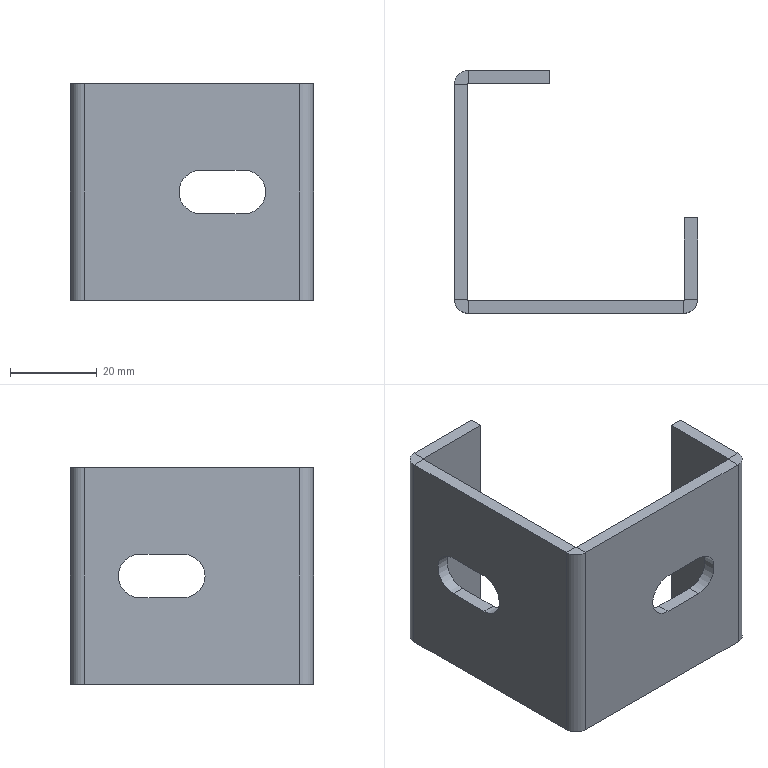Part | SolidWorks | features ICE 4, FlatPattern 1, SMBaseFlange 1, SheetMetal 1 | 1 solid | 39 faces | box 56 x 56 x 50 mm | volume 20650 mm3 | plane 28 | cylinder 11 | commonest cylinder face diameters 10 x5 0.4 x3 6.4 x3
STEP:
#1=CARTESIAN_POINT('',(3.,25.,0.));
#2=VERTEX_POINT('',#1);
#3=CARTESIAN_POINT('',(3.,30.,5.));
#4=VERTEX_POINT('',#3);
#5=CARTESIAN_POINT('',(3.,30.,0.));
#6=DIRECTION('',(-1.,0.,0.));
#7=DIRECTION('',(0.,-1.,0.));
#8=AXIS2_PLACEMENT_3D('',#5,#6,#7);
#9=CIRCLE('',#8,5.);
#10=EDGE_CURVE('',#2,#4,#9,.T.);
#11=ORIENTED_EDGE('',*,*,#10,.F.);
#12=CARTESIAN_POINT('',(0.,25.,0.));
#13=VERTEX_POINT('',#12);
#14=CARTESIAN_POINT('',(10.,25.,0.));
#15=DIRECTION('',(-1.,0.,0.));
#16=VECTOR('',#15,1000.);
#17=LINE('',#14,#16);
#18=EDGE_CURVE('',#2,#13,#17,.T.);
#19=ORIENTED_EDGE('',*,*,#18,.T.);
#20=CARTESIAN_POINT('',(0.,30.,5.));
#21=VERTEX_POINT('',#20);
#22=CARTESIAN_POINT('',(0.,30.,0.));
#23=DIRECTION('',(-1.,0.,0.));
#24=DIRECTION('',(0.,-1.,0.));
#25=AXIS2_PLACEMENT_3D('',#22,#23,#24);
#26=CIRCLE('',#25,5.);
#27=EDGE_CURVE('',#13,#21,#26,.T.);
#28=ORIENTED_EDGE('',*,*,#27,.T.);
#29=CARTESIAN_POINT('',(10.,30.,5.));
#30=DIRECTION('',(-1.,0.,0.));
#31=VECTOR('',#30,1000.);
#32=LINE('',#29,#31);
#33=EDGE_CURVE('',#4,#21,#32,.T.);
#34=ORIENTED_EDGE('',*,*,#33,.F.);
#35=EDGE_LOOP('',(#11,#19,#28,#34));
#36=FACE_OUTER_BOUND('',#35,.T.);
#37=CARTESIAN_POINT('',(10.,30.,0.));
#38=DIRECTION('',(-1.,0.,0.));
#39=DIRECTION('',(0.,-1.,0.));
#40=AXIS2_PLACEMENT_3D('',#37,#38,#39);
#41=CYLINDRICAL_SURFACE('',#40,5.);
#42=ADVANCED_FACE('',(#36),#41,.F.);
#43=CARTESIAN_POINT('',(52.8,0.,25.));
#44=VERTEX_POINT('',#43);
#45=CARTESIAN_POINT('',(52.8,3.,25.));
#46=VERTEX_POINT('',#45);
#47=CARTESIAN_POINT('',(52.8,0.,25.));
#48=DIRECTION('',(0.,1.,0.));
#49=VECTOR('',#48,1000.);
#50=LINE('',#47,#49);
#51=EDGE_CURVE('',#44,#46,#50,.T.);
#52=ORIENTED_EDGE('',*,*,#51,.F.);
#53=CARTESIAN_POINT('',(56.,3.2,25.));
#54=VERTEX_POINT('',#53);
#55=CARTESIAN_POINT('',(52.8,3.2,25.));
#56=DIRECTION('',(0.,0.,-1.));
#57=DIRECTION('',(1.,0.,0.));
#58=AXIS2_PLACEMENT_3D('',#55,#56,#57);
#59=CIRCLE('',#58,3.2);
#60=EDGE_CURVE('',#54,#44,#59,.T.);
#61=ORIENTED_EDGE('',*,*,#60,.F.);
#62=CARTESIAN_POINT('',(53.,3.2,25.));
#63=VERTEX_POINT('',#62);
#64=CARTESIAN_POINT('',(53.,3.2,25.));
#65=DIRECTION('',(1.,0.,0.));
#66=VECTOR('',#65,1000.);
#67=LINE('',#64,#66);
#68=EDGE_CURVE('',#63,#54,#67,.T.);
#69=ORIENTED_EDGE('',*,*,#68,.F.);
#70=CARTESIAN_POINT('',(52.8,3.2,25.));
#71=DIRECTION('',(0.,0.,-1.));
#72=DIRECTION('',(1.,0.,0.));
#73=AXIS2_PLACEMENT_3D('',#70,#71,#72);
#74=CIRCLE('',#73,0.2);
#75=EDGE_CURVE('',#63,#46,#74,.T.);
#76=ORIENTED_EDGE('',*,*,#75,.T.);
#77=EDGE_LOOP('',(#52,#61,#69,#76));
#78=FACE_OUTER_BOUND('',#77,.T.);
#79=CARTESIAN_POINT('',(52.8,0.,25.));
#80=DIRECTION('',(0.,0.,1.));
#81=DIRECTION('',(1.,0.,0.));
#82=AXIS2_PLACEMENT_3D('',#79,#80,#81);
#83=PLANE('',#82);
#84=ADVANCED_FACE('',(#78),#83,.T.);
#85=CARTESIAN_POINT('',(3.2,0.,25.));
#86=VERTEX_POINT('',#85);
#87=CARTESIAN_POINT('',(0.,0.,25.));
#88=DIRECTION('',(-1.,0.,0.));
#89=VECTOR('',#88,1000.);
#90=LINE('',#87,#89);
#91=EDGE_CURVE('',#44,#86,#90,.T.);
#92=ORIENTED_EDGE('',*,*,#91,.F.);
#93=ORIENTED_EDGE('',*,*,#51,.T.);
#94=CARTESIAN_POINT('',(3.2,3.,25.));
#95=VERTEX_POINT('',#94);
#96=CARTESIAN_POINT('',(0.,3.,25.));
#97=DIRECTION('',(-1.,0.,0.));
#98=VECTOR('',#97,1000.);
#99=LINE('',#96,#98);
#100=EDGE_CURVE('',#46,#95,#99,.T.);
#101=ORIENTED_EDGE('',*,*,#100,.T.);
#102=CARTESIAN_POINT('',(3.2,3.,25.));
#103=DIRECTION('',(0.,-1.,0.));
#104=VECTOR('',#103,1000.);
#105=LINE('',#102,#104);
#106=EDGE_CURVE('',#95,#86,#105,.T.);
#107=ORIENTED_EDGE('',*,*,#106,.T.);
#108=EDGE_LOOP('',(#92,#93,#101,#107));
#109=FACE_OUTER_BOUND('',#108,.T.);
#110=CARTESIAN_POINT('',(53.,3.2,25.));
#111=DIRECTION('',(0.,0.,1.));
#112=DIRECTION('',(1.,0.,0.));
#113=AXIS2_PLACEMENT_3D('',#110,#111,#112);
#114=PLANE('',#113);
#115=ADVANCED_FACE('',(#109),#114,.T.);
#116=CARTESIAN_POINT('',(56.,3.2,-25.));
#117=VERTEX_POINT('',#116);
#118=CARTESIAN_POINT('',(53.,3.2,-25.));
#119=VERTEX_POINT('',#118);
#120=CARTESIAN_POINT('',(56.,3.2,-25.));
#121=DIRECTION('',(-1.,0.,0.));
#122=VECTOR('',#121,1000.);
#123=LINE('',#120,#122);
#124=EDGE_CURVE('',#117,#119,#123,.T.);
#125=ORIENTED_EDGE('',*,*,#124,.F.);
#126=CARTESIAN_POINT('',(52.8,0.,-25.));
#127=VERTEX_POINT('',#126);
#128=CARTESIAN_POINT('',(52.8,3.2,-25.));
#129=DIRECTION('',(0.,0.,-1.));
#130=DIRECTION('',(1.,0.,0.));
#131=AXIS2_PLACEMENT_3D('',#128,#129,#130);
#132=CIRCLE('',#131,3.2);
#133=EDGE_CURVE('',#117,#127,#132,.T.);
#134=ORIENTED_EDGE('',*,*,#133,.T.);
#135=CARTESIAN_POINT('',(52.8,3.,-25.));
#136=VERTEX_POINT('',#135);
#137=CARTESIAN_POINT('',(52.8,3.,-25.));
#138=DIRECTION('',(0.,-1.,0.));
#139=VECTOR('',#138,1000.);
#140=LINE('',#137,#139);
#141=EDGE_CURVE('',#136,#127,#140,.T.);
#142=ORIENTED_EDGE('',*,*,#141,.F.);
#143=CARTESIAN_POINT('',(52.8,3.2,-25.));
#144=DIRECTION('',(0.,0.,-1.));
#145=DIRECTION('',(1.,0.,0.));
#146=AXIS2_PLACEMENT_3D('',#143,#144,#145);
#147=CIRCLE('',#146,0.2);
#148=EDGE_CURVE('',#119,#136,#147,.T.);
#149=ORIENTED_EDGE('',*,*,#148,.F.);
#150=EDGE_LOOP('',(#125,#134,#142,#149));
#151=FACE_OUTER_BOUND('',#150,.T.);
#152=CARTESIAN_POINT('',(56.,3.2,-25.));
#153=DIRECTION('',(0.,0.,-1.));
#154=DIRECTION('',(-1.,0.,0.));
#155=AXIS2_PLACEMENT_3D('',#152,#153,#154);
#156=PLANE('',#155);
#157=ADVANCED_FACE('',(#151),#156,.T.);
#158=CARTESIAN_POINT('',(56.,22.,-25.));
#159=VERTEX_POINT('',#158);
#160=CARTESIAN_POINT('',(56.,0.,-25.));
#161=DIRECTION('',(0.,-1.,0.));
#162=VECTOR('',#161,1000.);
#163=LINE('',#160,#162);
#164=EDGE_CURVE('',#159,#117,#163,.T.);
#165=ORIENTED_EDGE('',*,*,#164,.T.);
#166=ORIENTED_EDGE('',*,*,#124,.T.);
#167=CARTESIAN_POINT('',(53.,22.,-25.));
#168=VERTEX_POINT('',#167);
#169=CARTESIAN_POINT('',(53.,0.,-25.));
#170=DIRECTION('',(0.,-1.,0.));
#171=VECTOR('',#170,1000.);
#172=LINE('',#169,#171);
#173=EDGE_CURVE('',#168,#119,#172,.T.);
#174=ORIENTED_EDGE('',*,*,#173,.F.);
#175=CARTESIAN_POINT('',(53.,22.,-25.));
#176=DIRECTION('',(1.,0.,0.));
#177=VECTOR('',#176,1000.);
#178=LINE('',#175,#177);
#179=EDGE_CURVE('',#168,#159,#178,.T.);
#180=ORIENTED_EDGE('',*,*,#179,.T.);
#181=EDGE_LOOP('',(#165,#166,#174,#180));
#182=FACE_OUTER_BOUND('',#181,.T.);
#183=CARTESIAN_POINT('',(52.8,3.,-25.));
#184=DIRECTION('',(0.,0.,-1.));
#185=DIRECTION('',(-1.,0.,0.));
#186=AXIS2_PLACEMENT_3D('',#183,#184,#185);
#187=PLANE('',#186);
#188=ADVANCED_FACE('',(#182),#187,.T.);
#189=CARTESIAN_POINT('',(0.,3.2,25.));
#190=VERTEX_POINT('',#189);
#191=CARTESIAN_POINT('',(3.,3.2,25.));
#192=VERTEX_POINT('',#191);
#193=CARTESIAN_POINT('',(0.,3.2,25.));
#194=DIRECTION('',(1.,0.,0.));
#195=VECTOR('',#194,1000.);
#196=LINE('',#193,#195);
#197=EDGE_CURVE('',#190,#192,#196,.T.);
#198=ORIENTED_EDGE('',*,*,#197,.F.);
#199=CARTESIAN_POINT('',(3.2,3.2,25.));
#200=DIRECTION('',(0.,0.,-1.));
#201=DIRECTION('',(1.,0.,0.));
#202=AXIS2_PLACEMENT_3D('',#199,#200,#201);
#203=CIRCLE('',#202,3.2);
#204=EDGE_CURVE('',#86,#190,#203,.T.);
#205=ORIENTED_EDGE('',*,*,#204,.F.);
#206=ORIENTED_EDGE('',*,*,#106,.F.);
#207=CARTESIAN_POINT('',(3.2,3.2,25.));
#208=DIRECTION('',(0.,0.,-1.));
#209=DIRECTION('',(1.,0.,0.));
#210=AXIS2_PLACEMENT_3D('',#207,#208,#209);
#211=CIRCLE('',#210,0.2);
#212=EDGE_CURVE('',#95,#192,#211,.T.);
#213=ORIENTED_EDGE('',*,*,#212,.T.);
#214=EDGE_LOOP('',(#198,#205,#206,#213));
#215=FACE_OUTER_BOUND('',#214,.T.);
#216=CARTESIAN_POINT('',(0.,3.2,25.));
#217=DIRECTION('',(0.,0.,1.));
#218=DIRECTION('',(1.,0.,0.));
#219=AXIS2_PLACEMENT_3D('',#216,#217,#218);
#220=PLANE('',#219);
#221=ADVANCED_FACE('',(#215),#220,.T.);
#222=CARTESIAN_POINT('',(0.,52.8,25.));
#223=VERTEX_POINT('',#222);
#224=CARTESIAN_POINT('',(0.,56.,25.));
#225=DIRECTION('',(0.,1.,0.));
#226=VECTOR('',#225,1000.);
#227=LINE('',#224,#226);
#228=EDGE_CURVE('',#190,#223,#227,.T.);
#229=ORIENTED_EDGE('',*,*,#228,.F.);
#230=ORIENTED_EDGE('',*,*,#197,.T.);
#231=CARTESIAN_POINT('',(3.,52.8,25.));
#232=VERTEX_POINT('',#231);
#233=CARTESIAN_POINT('',(3.,56.,25.));
#234=DIRECTION('',(0.,1.,0.));
#235=VECTOR('',#234,1000.);
#236=LINE('',#233,#235);
#237=EDGE_CURVE('',#192,#232,#236,.T.);
#238=ORIENTED_EDGE('',*,*,#237,.T.);
#239=CARTESIAN_POINT('',(3.,52.8,25.));
#240=DIRECTION('',(-1.,0.,0.));
#241=VECTOR('',#240,1000.);
#242=LINE('',#239,#241);
#243=EDGE_CURVE('',#232,#223,#242,.T.);
#244=ORIENTED_EDGE('',*,*,#243,.T.);
#245=EDGE_LOOP('',(#229,#230,#238,#244));
#246=FACE_OUTER_BOUND('',#245,.T.);
#247=CARTESIAN_POINT('',(3.2,3.,25.));
#248=DIRECTION('',(0.,0.,1.));
#249=DIRECTION('',(1.,0.,0.));
#250=AXIS2_PLACEMENT_3D('',#247,#248,#249);
#251=PLANE('',#250);
#252=ADVANCED_FACE('',(#246),#251,.T.);
#253=CARTESIAN_POINT('',(3.2,0.,-25.));
#254=VERTEX_POINT('',#253);
#255=CARTESIAN_POINT('',(3.2,3.,-25.));
#256=VERTEX_POINT('',#255);
#257=CARTESIAN_POINT('',(3.2,0.,-25.));
#258=DIRECTION('',(0.,1.,0.));
#259=VECTOR('',#258,1000.);
#260=LINE('',#257,#259);
#261=EDGE_CURVE('',#254,#256,#260,.T.);
#262=ORIENTED_EDGE('',*,*,#261,.F.);
#263=CARTESIAN_POINT('',(0.,3.2,-25.));
#264=VERTEX_POINT('',#263);
#265=CARTESIAN_POINT('',(3.2,3.2,-25.));
#266=DIRECTION('',(0.,0.,-1.));
#267=DIRECTION('',(1.,0.,0.));
#268=AXIS2_PLACEMENT_3D('',#265,#266,#267);
#269=CIRCLE('',#268,3.2);
#270=EDGE_CURVE('',#254,#264,#269,.T.);
#271=ORIENTED_EDGE('',*,*,#270,.T.);
#272=CARTESIAN_POINT('',(3.,3.2,-25.));
#273=VERTEX_POINT('',#272);
#274=CARTESIAN_POINT('',(3.,3.2,-25.));
#275=DIRECTION('',(-1.,0.,0.));
#276=VECTOR('',#275,1000.);
#277=LINE('',#274,#276);
#278=EDGE_CURVE('',#273,#264,#277,.T.);
#279=ORIENTED_EDGE('',*,*,#278,.F.);
#280=CARTESIAN_POINT('',(3.2,3.2,-25.));
#281=DIRECTION('',(0.,0.,-1.));
#282=DIRECTION('',(1.,0.,0.));
#283=AXIS2_PLACEMENT_3D('',#280,#281,#282);
#284=CIRCLE('',#283,0.2);
#285=EDGE_CURVE('',#256,#273,#284,.T.);
#286=ORIENTED_EDGE('',*,*,#285,.F.);
#287=EDGE_LOOP('',(#262,#271,#279,#286));
#288=FACE_OUTER_BOUND('',#287,.T.);
#289=CARTESIAN_POINT('',(3.2,0.,-25.));
#290=DIRECTION('',(0.,0.,-1.));
#291=DIRECTION('',(-1.,0.,0.));
#292=AXIS2_PLACEMENT_3D('',#289,#290,#291);
#293=PLANE('',#292);
#294=ADVANCED_FACE('',(#288),#293,.T.);
#295=CARTESIAN_POINT('',(0.,0.,-25.));
#296=DIRECTION('',(-1.,0.,0.));
#297=VECTOR('',#296,1000.);
#298=LINE('',#295,#297);
#299=EDGE_CURVE('',#127,#254,#298,.T.);
#300=ORIENTED_EDGE('',*,*,#299,.T.);
#301=ORIENTED_EDGE('',*,*,#261,.T.);
#302=CARTESIAN_POINT('',(0.,3.,-25.));
#303=DIRECTION('',(-1.,0.,0.));
#304=VECTOR('',#303,1000.);
#305=LINE('',#302,#304);
#306=EDGE_CURVE('',#136,#256,#305,.T.);
#307=ORIENTED_EDGE('',*,*,#306,.F.);
#308=ORIENTED_EDGE('',*,*,#141,.T.);
#309=EDGE_LOOP('',(#300,#301,#307,#308));
#310=FACE_OUTER_BOUND('',#309,.T.);
#311=CARTESIAN_POINT('',(3.,3.2,-25.));
#312=DIRECTION('',(0.,0.,-1.));
#313=DIRECTION('',(-1.,0.,0.));
#314=AXIS2_PLACEMENT_3D('',#311,#312,#313);
#315=PLANE('',#314);
#316=ADVANCED_FACE('',(#310),#315,.T.);
#317=CARTESIAN_POINT('',(3.2,56.,25.));
#318=VERTEX_POINT('',#317);
#319=CARTESIAN_POINT('',(3.2,53.,25.));
#320=VERTEX_POINT('',#319);
#321=CARTESIAN_POINT('',(3.2,56.,25.));
#322=DIRECTION('',(0.,-1.,0.));
#323=VECTOR('',#322,1000.);
#324=LINE('',#321,#323);
#325=EDGE_CURVE('',#318,#320,#324,.T.);
#326=ORIENTED_EDGE('',*,*,#325,.F.);
#327=CARTESIAN_POINT('',(3.2,52.8,25.));
#328=DIRECTION('',(0.,0.,-1.));
#329=DIRECTION('',(1.,0.,0.));
#330=AXIS2_PLACEMENT_3D('',#327,#328,#329);
#331=CIRCLE('',#330,3.2);
#332=EDGE_CURVE('',#223,#318,#331,.T.);
#333=ORIENTED_EDGE('',*,*,#332,.F.);
#334=ORIENTED_EDGE('',*,*,#243,.F.);
#335=CARTESIAN_POINT('',(3.2,52.8,25.));
#336=DIRECTION('',(0.,0.,-1.));
#337=DIRECTION('',(1.,0.,0.));
#338=AXIS2_PLACEMENT_3D('',#335,#336,#337);
#339=CIRCLE('',#338,0.2);
#340=EDGE_CURVE('',#232,#320,#339,.T.);
#341=ORIENTED_EDGE('',*,*,#340,.T.);
#342=EDGE_LOOP('',(#326,#333,#334,#341));
#343=FACE_OUTER_BOUND('',#342,.T.);
#344=CARTESIAN_POINT('',(3.2,56.,25.));
#345=DIRECTION('',(0.,0.,1.));
#346=DIRECTION('',(1.,0.,0.));
#347=AXIS2_PLACEMENT_3D('',#344,#345,#346);
#348=PLANE('',#347);
#349=ADVANCED_FACE('',(#343),#348,.T.);
#350=CARTESIAN_POINT('',(22.,56.,25.));
#351=VERTEX_POINT('',#350);
#352=CARTESIAN_POINT('',(0.,56.,25.));
#353=DIRECTION('',(1.,0.,0.));
#354=VECTOR('',#353,1000.);
#355=LINE('',#352,#354);
#356=EDGE_CURVE('',#318,#351,#355,.T.);
#357=ORIENTED_EDGE('',*,*,#356,.F.);
#358=ORIENTED_EDGE('',*,*,#325,.T.);
#359=CARTESIAN_POINT('',(22.,53.,25.));
#360=VERTEX_POINT('',#359);
#361=CARTESIAN_POINT('',(0.,53.,25.));
#362=DIRECTION('',(1.,0.,0.));
#363=VECTOR('',#362,1000.);
#364=LINE('',#361,#363);
#365=EDGE_CURVE('',#320,#360,#364,.T.);
#366=ORIENTED_EDGE('',*,*,#365,.T.);
#367=CARTESIAN_POINT('',(22.,56.,25.));
#368=DIRECTION('',(0.,-1.,0.));
#369=VECTOR('',#368,1000.);
#370=LINE('',#367,#369);
#371=EDGE_CURVE('',#351,#360,#370,.T.);
#372=ORIENTED_EDGE('',*,*,#371,.F.);
#373=EDGE_LOOP('',(#357,#358,#366,#372));
#374=FACE_OUTER_BOUND('',#373,.T.);
#375=CARTESIAN_POINT('',(3.,52.8,25.));
#376=DIRECTION('',(0.,0.,1.));
#377=DIRECTION('',(1.,0.,0.));
#378=AXIS2_PLACEMENT_3D('',#375,#376,#377);
#379=PLANE('',#378);
#380=ADVANCED_FACE('',(#374),#379,.T.);
#381=CARTESIAN_POINT('',(0.,52.8,-25.));
#382=VERTEX_POINT('',#381);
#383=CARTESIAN_POINT('',(3.,52.8,-25.));
#384=VERTEX_POINT('',#383);
#385=CARTESIAN_POINT('',(0.,52.8,-25.));
#386=DIRECTION('',(1.,0.,0.));
#387=VECTOR('',#386,1000.);
#388=LINE('',#385,#387);
#389=EDGE_CURVE('',#382,#384,#388,.T.);
#390=ORIENTED_EDGE('',*,*,#389,.F.);
#391=CARTESIAN_POINT('',(3.2,56.,-25.));
#392=VERTEX_POINT('',#391);
#393=CARTESIAN_POINT('',(3.2,52.8,-25.));
#394=DIRECTION('',(0.,0.,-1.));
#395=DIRECTION('',(1.,0.,0.));
#396=AXIS2_PLACEMENT_3D('',#393,#394,#395);
#397=CIRCLE('',#396,3.2);
#398=EDGE_CURVE('',#382,#392,#397,.T.);
#399=ORIENTED_EDGE('',*,*,#398,.T.);
#400=CARTESIAN_POINT('',(3.2,53.,-25.));
#401=VERTEX_POINT('',#400);
#402=CARTESIAN_POINT('',(3.2,53.,-25.));
#403=DIRECTION('',(0.,1.,0.));
#404=VECTOR('',#403,1000.);
#405=LINE('',#402,#404);
#406=EDGE_CURVE('',#401,#392,#405,.T.);
#407=ORIENTED_EDGE('',*,*,#406,.F.);
#408=CARTESIAN_POINT('',(3.2,52.8,-25.));
#409=DIRECTION('',(0.,0.,-1.));
#410=DIRECTION('',(1.,0.,0.));
#411=AXIS2_PLACEMENT_3D('',#408,#409,#410);
#412=CIRCLE('',#411,0.2);
#413=EDGE_CURVE('',#384,#401,#412,.T.);
#414=ORIENTED_EDGE('',*,*,#413,.F.);
#415=EDGE_LOOP('',(#390,#399,#407,#414));
#416=FACE_OUTER_BOUND('',#415,.T.);
#417=CARTESIAN_POINT('',(0.,52.8,-25.));
#418=DIRECTION('',(0.,0.,-1.));
#419=DIRECTION('',(-1.,0.,0.));
#420=AXIS2_PLACEMENT_3D('',#417,#418,#419);
#421=PLANE('',#420);
#422=ADVANCED_FACE('',(#416),#421,.T.);
#423=CARTESIAN_POINT('',(0.,56.,-25.));
#424=DIRECTION('',(0.,1.,0.));
#425=VECTOR('',#424,1000.);
#426=LINE('',#423,#425);
#427=EDGE_CURVE('',#264,#382,#426,.T.);
#428=ORIENTED_EDGE('',*,*,#427,.T.);
#429=ORIENTED_EDGE('',*,*,#389,.T.);
#430=CARTESIAN_POINT('',(3.,56.,-25.));
#431=DIRECTION('',(0.,1.,0.));
#432=VECTOR('',#431,1000.);
#433=LINE('',#430,#432);
#434=EDGE_CURVE('',#273,#384,#433,.T.);
#435=ORIENTED_EDGE('',*,*,#434,.F.);
#436=ORIENTED_EDGE('',*,*,#278,.T.);
#437=EDGE_LOOP('',(#428,#429,#435,#436));
#438=FACE_OUTER_BOUND('',#437,.T.);
#439=CARTESIAN_POINT('',(3.2,53.,-25.));
#440=DIRECTION('',(0.,0.,-1.));
#441=DIRECTION('',(-1.,0.,0.));
#442=AXIS2_PLACEMENT_3D('',#439,#440,#441);
#443=PLANE('',#442);
#444=ADVANCED_FACE('',(#438),#443,.T.);
#445=CARTESIAN_POINT('',(22.,53.,-25.));
#446=VERTEX_POINT('',#445);
#447=CARTESIAN_POINT('',(0.,53.,-25.));
#448=DIRECTION('',(1.,0.,0.));
#449=VECTOR('',#448,1000.);
#450=LINE('',#447,#449);
#451=EDGE_CURVE('',#401,#446,#450,.T.);
#452=ORIENTED_EDGE('',*,*,#451,.T.);
#453=CARTESIAN_POINT('',(22.,53.,25.));
#454=DIRECTION('',(0.,0.,-1.));
#455=VECTOR('',#454,1000.);
#456=LINE('',#453,#455);
#457=EDGE_CURVE('',#360,#446,#456,.T.);
#458=ORIENTED_EDGE('',*,*,#457,.F.);
#459=ORIENTED_EDGE('',*,*,#365,.F.);
#460=CARTESIAN_POINT('',(3.2,53.,25.));
#461=DIRECTION('',(0.,0.,-1.));
#462=VECTOR('',#461,1000.);
#463=LINE('',#460,#462);
#464=EDGE_CURVE('',#320,#401,#463,.T.);
#465=ORIENTED_EDGE('',*,*,#464,.T.);
#466=EDGE_LOOP('',(#452,#458,#459,#465));
#467=FACE_OUTER_BOUND('',#466,.T.);
#468=CARTESIAN_POINT('',(0.,53.,25.));
#469=DIRECTION('',(0.,1.,0.));
#470=DIRECTION('',(0.,0.,1.));
#471=AXIS2_PLACEMENT_3D('',#468,#469,#470);
#472=PLANE('',#471);
#473=ADVANCED_FACE('',(#467),#472,.F.);
#474=CARTESIAN_POINT('',(22.,56.,-25.));
#475=VERTEX_POINT('',#474);
#476=CARTESIAN_POINT('',(22.,56.,-25.));
#477=DIRECTION('',(0.,-1.,0.));
#478=VECTOR('',#477,1000.);
#479=LINE('',#476,#478);
#480=EDGE_CURVE('',#475,#446,#479,.T.);
#481=ORIENTED_EDGE('',*,*,#480,.F.);
#482=CARTESIAN_POINT('',(22.,56.,25.));
#483=DIRECTION('',(0.,0.,-1.));
#484=VECTOR('',#483,1000.);
#485=LINE('',#482,#484);
#486=EDGE_CURVE('',#351,#475,#485,.T.);
#487=ORIENTED_EDGE('',*,*,#486,.F.);
#488=ORIENTED_EDGE('',*,*,#371,.T.);
#489=ORIENTED_EDGE('',*,*,#457,.T.);
#490=EDGE_LOOP('',(#481,#487,#488,#489));
#491=FACE_OUTER_BOUND('',#490,.T.);
#492=CARTESIAN_POINT('',(22.,56.,25.));
#493=DIRECTION('',(1.,0.,0.));
#494=DIRECTION('',(0.,0.,-1.));
#495=AXIS2_PLACEMENT_3D('',#492,#493,#494);
#496=PLANE('',#495);
#497=ADVANCED_FACE('',(#491),#496,.T.);
#498=CARTESIAN_POINT('',(0.,56.,-25.));
#499=DIRECTION('',(1.,0.,0.));
#500=VECTOR('',#499,1000.);
#501=LINE('',#498,#500);
#502=EDGE_CURVE('',#392,#475,#501,.T.);
#503=ORIENTED_EDGE('',*,*,#502,.F.);
#504=CARTESIAN_POINT('',(3.2,56.,25.));
#505=DIRECTION('',(0.,0.,-1.));
#506=VECTOR('',#505,1000.);
#507=LINE('',#504,#506);
#508=EDGE_CURVE('',#318,#392,#507,.T.);
#509=ORIENTED_EDGE('',*,*,#508,.F.);
#510=ORIENTED_EDGE('',*,*,#356,.T.);
#511=ORIENTED_EDGE('',*,*,#486,.T.);
#512=EDGE_LOOP('',(#503,#509,#510,#511));
#513=FACE_OUTER_BOUND('',#512,.T.);
#514=CARTESIAN_POINT('',(0.,56.,25.));
#515=DIRECTION('',(0.,1.,0.));
#516=DIRECTION('',(0.,0.,1.));
#517=AXIS2_PLACEMENT_3D('',#514,#515,#516);
#518=PLANE('',#517);
#519=ADVANCED_FACE('',(#513),#518,.T.);
#520=ORIENTED_EDGE('',*,*,#398,.F.);
#521=CARTESIAN_POINT('',(0.,52.8,25.));
#522=DIRECTION('',(0.,0.,-1.));
#523=VECTOR('',#522,1000.);
#524=LINE('',#521,#523);
#525=EDGE_CURVE('',#223,#382,#524,.T.);
#526=ORIENTED_EDGE('',*,*,#525,.F.);
#527=ORIENTED_EDGE('',*,*,#332,.T.);
#528=ORIENTED_EDGE('',*,*,#508,.T.);
#529=EDGE_LOOP('',(#520,#526,#527,#528));
#530=FACE_OUTER_BOUND('',#529,.T.);
#531=CARTESIAN_POINT('',(3.2,52.8,25.));
#532=DIRECTION('',(0.,0.,-1.));
#533=DIRECTION('',(-1.,0.,0.));
#534=AXIS2_PLACEMENT_3D('',#531,#532,#533);
#535=CYLINDRICAL_SURFACE('',#534,3.2);
#536=ADVANCED_FACE('',(#530),#535,.T.);
#537=CARTESIAN_POINT('',(0.,40.,5.));
#538=VERTEX_POINT('',#537);
#539=CARTESIAN_POINT('',(0.,40.,-5.));
#540=VERTEX_POINT('',#539);
#541=CARTESIAN_POINT('',(0.,40.,0.));
#542=DIRECTION('',(-1.,0.,0.));
#543=DIRECTION('',(0.,-1.,0.));
#544=AXIS2_PLACEMENT_3D('',#541,#542,#543);
#545=CIRCLE('',#544,5.);
#546=EDGE_CURVE('',#538,#540,#545,.T.);
#547=ORIENTED_EDGE('',*,*,#546,.F.);
#548=CARTESIAN_POINT('',(0.,40.,5.));
#549=DIRECTION('',(0.,1.,0.));
#550=VECTOR('',#549,1000.);
#551=LINE('',#548,#550);
#552=EDGE_CURVE('',#21,#538,#551,.T.);
#553=ORIENTED_EDGE('',*,*,#552,.F.);
#554=ORIENTED_EDGE('',*,*,#27,.F.);
#555=CARTESIAN_POINT('',(0.,30.,-5.));
#556=VERTEX_POINT('',#555);
#557=CARTESIAN_POINT('',(0.,30.,0.));
#558=DIRECTION('',(-1.,0.,0.));
#559=DIRECTION('',(0.,-1.,0.));
#560=AXIS2_PLACEMENT_3D('',#557,#558,#559);
#561=CIRCLE('',#560,5.);
#562=EDGE_CURVE('',#556,#13,#561,.T.);
#563=ORIENTED_EDGE('',*,*,#562,.F.);
#564=CARTESIAN_POINT('',(0.,40.,-5.));
#565=DIRECTION('',(0.,-1.,0.));
#566=VECTOR('',#565,1000.);
#567=LINE('',#564,#566);
#568=EDGE_CURVE('',#540,#556,#567,.T.);
#569=ORIENTED_EDGE('',*,*,#568,.F.);
#570=EDGE_LOOP('',(#547,#553,#554,#563,#569));
#571=FACE_BOUND('',#570,.T.);
#572=ORIENTED_EDGE('',*,*,#427,.F.);
#573=CARTESIAN_POINT('',(0.,3.2,25.));
#574=DIRECTION('',(0.,0.,-1.));
#575=VECTOR('',#574,1000.);
#576=LINE('',#573,#575);
#577=EDGE_CURVE('',#190,#264,#576,.T.);
#578=ORIENTED_EDGE('',*,*,#577,.F.);
#579=ORIENTED_EDGE('',*,*,#228,.T.);
#580=ORIENTED_EDGE('',*,*,#525,.T.);
#581=EDGE_LOOP('',(#572,#578,#579,#580));
#582=FACE_OUTER_BOUND('',#581,.T.);
#583=CARTESIAN_POINT('',(0.,56.,25.));
#584=DIRECTION('',(-1.,0.,0.));
#585=DIRECTION('',(0.,-1.,0.));
#586=AXIS2_PLACEMENT_3D('',#583,#584,#585);
#587=PLANE('',#586);
#588=ADVANCED_FACE('',(#571,#582),#587,.T.);
#589=ORIENTED_EDGE('',*,*,#270,.F.);
#590=CARTESIAN_POINT('',(3.2,0.,25.));
#591=DIRECTION('',(0.,0.,-1.));
#592=VECTOR('',#591,1000.);
#593=LINE('',#590,#592);
#594=EDGE_CURVE('',#86,#254,#593,.T.);
#595=ORIENTED_EDGE('',*,*,#594,.F.);
#596=ORIENTED_EDGE('',*,*,#204,.T.);
#597=ORIENTED_EDGE('',*,*,#577,.T.);
#598=EDGE_LOOP('',(#589,#595,#596,#597));
#599=FACE_OUTER_BOUND('',#598,.T.);
#600=CARTESIAN_POINT('',(3.2,3.2,25.));
#601=DIRECTION('',(0.,0.,-1.));
#602=DIRECTION('',(-1.,0.,0.));
#603=AXIS2_PLACEMENT_3D('',#600,#601,#602);
#604=CYLINDRICAL_SURFACE('',#603,3.2);
#605=ADVANCED_FACE('',(#599),#604,.T.);
#606=CARTESIAN_POINT('',(40.,0.,-5.));
#607=VERTEX_POINT('',#606);
#608=CARTESIAN_POINT('',(40.,0.,5.));
#609=VERTEX_POINT('',#608);
#610=CARTESIAN_POINT('',(40.,0.,0.));
#611=DIRECTION('',(0.,-1.,0.));
#612=DIRECTION('',(0.,0.,-1.));
#613=AXIS2_PLACEMENT_3D('',#610,#611,#612);
#614=CIRCLE('',#613,5.);
#615=EDGE_CURVE('',#607,#609,#614,.T.);
#616=ORIENTED_EDGE('',*,*,#615,.F.);
#617=CARTESIAN_POINT('',(30.,0.,-5.));
#618=VERTEX_POINT('',#617);
#619=CARTESIAN_POINT('',(40.,0.,-5.));
#620=DIRECTION('',(1.,0.,0.));
#621=VECTOR('',#620,1000.);
#622=LINE('',#619,#621);
#623=EDGE_CURVE('',#618,#607,#622,.T.);
#624=ORIENTED_EDGE('',*,*,#623,.F.);
#625=CARTESIAN_POINT('',(30.,0.,5.));
#626=VERTEX_POINT('',#625);
#627=CARTESIAN_POINT('',(30.,0.,0.));
#628=DIRECTION('',(0.,-1.,0.));
#629=DIRECTION('',(0.,0.,-1.));
#630=AXIS2_PLACEMENT_3D('',#627,#628,#629);
#631=CIRCLE('',#630,5.);
#632=EDGE_CURVE('',#626,#618,#631,.T.);
#633=ORIENTED_EDGE('',*,*,#632,.F.);
#634=CARTESIAN_POINT('',(40.,0.,5.));
#635=DIRECTION('',(-1.,0.,0.));
#636=VECTOR('',#635,1000.);
#637=LINE('',#634,#636);
#638=EDGE_CURVE('',#609,#626,#637,.T.);
#639=ORIENTED_EDGE('',*,*,#638,.F.);
#640=EDGE_LOOP('',(#616,#624,#633,#639));
#641=FACE_BOUND('',#640,.T.);
#642=ORIENTED_EDGE('',*,*,#299,.F.);
#643=CARTESIAN_POINT('',(52.8,0.,25.));
#644=DIRECTION('',(0.,0.,-1.));
#645=VECTOR('',#644,1000.);
#646=LINE('',#643,#645);
#647=EDGE_CURVE('',#44,#127,#646,.T.);
#648=ORIENTED_EDGE('',*,*,#647,.F.);
#649=ORIENTED_EDGE('',*,*,#91,.T.);
#650=ORIENTED_EDGE('',*,*,#594,.T.);
#651=EDGE_LOOP('',(#642,#648,#649,#650));
#652=FACE_OUTER_BOUND('',#651,.T.);
#653=CARTESIAN_POINT('',(0.,0.,25.));
#654=DIRECTION('',(0.,-1.,0.));
#655=DIRECTION('',(0.,0.,-1.));
#656=AXIS2_PLACEMENT_3D('',#653,#654,#655);
#657=PLANE('',#656);
#658=ADVANCED_FACE('',(#641,#652),#657,.T.);
#659=ORIENTED_EDGE('',*,*,#133,.F.);
#660=CARTESIAN_POINT('',(56.,3.2,25.));
#661=DIRECTION('',(0.,0.,-1.));
#662=VECTOR('',#661,1000.);
#663=LINE('',#660,#662);
#664=EDGE_CURVE('',#54,#117,#663,.T.);
#665=ORIENTED_EDGE('',*,*,#664,.F.);
#666=ORIENTED_EDGE('',*,*,#60,.T.);
#667=ORIENTED_EDGE('',*,*,#647,.T.);
#668=EDGE_LOOP('',(#659,#665,#666,#667));
#669=FACE_OUTER_BOUND('',#668,.T.);
#670=CARTESIAN_POINT('',(52.8,3.2,25.));
#671=DIRECTION('',(0.,0.,-1.));
#672=DIRECTION('',(-1.,0.,0.));
#673=AXIS2_PLACEMENT_3D('',#670,#671,#672);
#674=CYLINDRICAL_SURFACE('',#673,3.2);
#675=ADVANCED_FACE('',(#669),#674,.T.);
#676=ORIENTED_EDGE('',*,*,#164,.F.);
#677=CARTESIAN_POINT('',(56.,22.,25.));
#678=VERTEX_POINT('',#677);
#679=CARTESIAN_POINT('',(56.,22.,25.));
#680=DIRECTION('',(0.,0.,-1.));
#681=VECTOR('',#680,1000.);
#682=LINE('',#679,#681);
#683=EDGE_CURVE('',#678,#159,#682,.T.);
#684=ORIENTED_EDGE('',*,*,#683,.F.);
#685=CARTESIAN_POINT('',(56.,0.,25.));
#686=DIRECTION('',(0.,-1.,0.));
#687=VECTOR('',#686,1000.);
#688=LINE('',#685,#687);
#689=EDGE_CURVE('',#678,#54,#688,.T.);
#690=ORIENTED_EDGE('',*,*,#689,.T.);
#691=ORIENTED_EDGE('',*,*,#664,.T.);
#692=EDGE_LOOP('',(#676,#684,#690,#691));
#693=FACE_OUTER_BOUND('',#692,.T.);
#694=CARTESIAN_POINT('',(56.,0.,25.));
#695=DIRECTION('',(1.,0.,0.));
#696=DIRECTION('',(0.,0.,-1.));
#697=AXIS2_PLACEMENT_3D('',#694,#695,#696);
#698=PLANE('',#697);
#699=ADVANCED_FACE('',(#693),#698,.T.);
#700=ORIENTED_EDGE('',*,*,#179,.F.);
#701=CARTESIAN_POINT('',(53.,22.,25.));
#702=VERTEX_POINT('',#701);
#703=CARTESIAN_POINT('',(53.,22.,25.));
#704=DIRECTION('',(0.,0.,-1.));
#705=VECTOR('',#704,1000.);
#706=LINE('',#703,#705);
#707=EDGE_CURVE('',#702,#168,#706,.T.);
#708=ORIENTED_EDGE('',*,*,#707,.F.);
#709=CARTESIAN_POINT('',(53.,22.,25.));
#710=DIRECTION('',(1.,0.,0.));
#711=VECTOR('',#710,1000.);
#712=LINE('',#709,#711);
#713=EDGE_CURVE('',#702,#678,#712,.T.);
#714=ORIENTED_EDGE('',*,*,#713,.T.);
#715=ORIENTED_EDGE('',*,*,#683,.T.);
#716=EDGE_LOOP('',(#700,#708,#714,#715));
#717=FACE_OUTER_BOUND('',#716,.T.);
#718=CARTESIAN_POINT('',(53.,22.,25.));
#719=DIRECTION('',(0.,1.,0.));
#720=DIRECTION('',(0.,0.,1.));
#721=AXIS2_PLACEMENT_3D('',#718,#719,#720);
#722=PLANE('',#721);
#723=ADVANCED_FACE('',(#717),#722,.T.);
#724=ORIENTED_EDGE('',*,*,#173,.T.);
#725=CARTESIAN_POINT('',(53.,3.2,25.));
#726=DIRECTION('',(0.,0.,-1.));
#727=VECTOR('',#726,1000.);
#728=LINE('',#725,#727);
#729=EDGE_CURVE('',#63,#119,#728,.T.);
#730=ORIENTED_EDGE('',*,*,#729,.F.);
#731=CARTESIAN_POINT('',(53.,0.,25.));
#732=DIRECTION('',(0.,-1.,0.));
#733=VECTOR('',#732,1000.);
#734=LINE('',#731,#733);
#735=EDGE_CURVE('',#702,#63,#734,.T.);
#736=ORIENTED_EDGE('',*,*,#735,.F.);
#737=ORIENTED_EDGE('',*,*,#707,.T.);
#738=EDGE_LOOP('',(#724,#730,#736,#737));
#739=FACE_OUTER_BOUND('',#738,.T.);
#740=CARTESIAN_POINT('',(53.,0.,25.));
#741=DIRECTION('',(1.,0.,0.));
#742=DIRECTION('',(0.,0.,-1.));
#743=AXIS2_PLACEMENT_3D('',#740,#741,#742);
#744=PLANE('',#743);
#745=ADVANCED_FACE('',(#739),#744,.F.);
#746=ORIENTED_EDGE('',*,*,#148,.T.);
#747=CARTESIAN_POINT('',(52.8,3.,25.));
#748=DIRECTION('',(0.,0.,-1.));
#749=VECTOR('',#748,1000.);
#750=LINE('',#747,#749);
#751=EDGE_CURVE('',#46,#136,#750,.T.);
#752=ORIENTED_EDGE('',*,*,#751,.F.);
#753=ORIENTED_EDGE('',*,*,#75,.F.);
#754=ORIENTED_EDGE('',*,*,#729,.T.);
#755=EDGE_LOOP('',(#746,#752,#753,#754));
#756=FACE_OUTER_BOUND('',#755,.T.);
#757=CARTESIAN_POINT('',(52.8,3.2,25.));
#758=DIRECTION('',(0.,0.,-1.));
#759=DIRECTION('',(-1.,0.,0.));
#760=AXIS2_PLACEMENT_3D('',#757,#758,#759);
#761=CYLINDRICAL_SURFACE('',#760,0.2);
#762=ADVANCED_FACE('',(#756),#761,.F.);
#763=CARTESIAN_POINT('',(30.,3.,-5.));
#764=VERTEX_POINT('',#763);
#765=CARTESIAN_POINT('',(40.,3.,-5.));
#766=VERTEX_POINT('',#765);
#767=CARTESIAN_POINT('',(0.,3.,-5.));
#768=DIRECTION('',(1.,0.,0.));
#769=VECTOR('',#768,1000.);
#770=LINE('',#767,#769);
#771=EDGE_CURVE('',#764,#766,#770,.T.);
#772=ORIENTED_EDGE('',*,*,#771,.T.);
#773=CARTESIAN_POINT('',(40.,3.,5.));
#774=VERTEX_POINT('',#773);
#775=CARTESIAN_POINT('',(40.,3.,0.));
#776=DIRECTION('',(0.,-1.,0.));
#777=DIRECTION('',(0.,0.,-1.));
#778=AXIS2_PLACEMENT_3D('',#775,#776,#777);
#779=CIRCLE('',#778,5.);
#780=EDGE_CURVE('',#766,#774,#779,.T.);
#781=ORIENTED_EDGE('',*,*,#780,.T.);
#782=CARTESIAN_POINT('',(30.,3.,5.));
#783=VERTEX_POINT('',#782);
#784=CARTESIAN_POINT('',(0.,3.,5.));
#785=DIRECTION('',(-1.,0.,0.));
#786=VECTOR('',#785,1000.);
#787=LINE('',#784,#786);
#788=EDGE_CURVE('',#774,#783,#787,.T.);
#789=ORIENTED_EDGE('',*,*,#788,.T.);
#790=CARTESIAN_POINT('',(30.,3.,0.));
#791=DIRECTION('',(0.,-1.,0.));
#792=DIRECTION('',(0.,0.,-1.));
#793=AXIS2_PLACEMENT_3D('',#790,#791,#792);
#794=CIRCLE('',#793,5.);
#795=EDGE_CURVE('',#783,#764,#794,.T.);
#796=ORIENTED_EDGE('',*,*,#795,.T.);
#797=EDGE_LOOP('',(#772,#781,#789,#796));
#798=FACE_BOUND('',#797,.T.);
#799=ORIENTED_EDGE('',*,*,#306,.T.);
#800=CARTESIAN_POINT('',(3.2,3.,25.));
#801=DIRECTION('',(0.,0.,-1.));
#802=VECTOR('',#801,1000.);
#803=LINE('',#800,#802);
#804=EDGE_CURVE('',#95,#256,#803,.T.);
#805=ORIENTED_EDGE('',*,*,#804,.F.);
#806=ORIENTED_EDGE('',*,*,#100,.F.);
#807=ORIENTED_EDGE('',*,*,#751,.T.);
#808=EDGE_LOOP('',(#799,#805,#806,#807));
#809=FACE_OUTER_BOUND('',#808,.T.);
#810=CARTESIAN_POINT('',(0.,3.,25.));
#811=DIRECTION('',(0.,-1.,0.));
#812=DIRECTION('',(0.,0.,-1.));
#813=AXIS2_PLACEMENT_3D('',#810,#811,#812);
#814=PLANE('',#813);
#815=ADVANCED_FACE('',(#798,#809),#814,.F.);
#816=ORIENTED_EDGE('',*,*,#285,.T.);
#817=CARTESIAN_POINT('',(3.,3.2,25.));
#818=DIRECTION('',(0.,0.,-1.));
#819=VECTOR('',#818,1000.);
#820=LINE('',#817,#819);
#821=EDGE_CURVE('',#192,#273,#820,.T.);
#822=ORIENTED_EDGE('',*,*,#821,.F.);
#823=ORIENTED_EDGE('',*,*,#212,.F.);
#824=ORIENTED_EDGE('',*,*,#804,.T.);
#825=EDGE_LOOP('',(#816,#822,#823,#824));
#826=FACE_OUTER_BOUND('',#825,.T.);
#827=CARTESIAN_POINT('',(3.2,3.2,25.));
#828=DIRECTION('',(0.,0.,-1.));
#829=DIRECTION('',(-1.,0.,0.));
#830=AXIS2_PLACEMENT_3D('',#827,#828,#829);
#831=CYLINDRICAL_SURFACE('',#830,0.2);
#832=ADVANCED_FACE('',(#826),#831,.F.);
#833=CARTESIAN_POINT('',(3.,40.,5.));
#834=VERTEX_POINT('',#833);
#835=CARTESIAN_POINT('',(3.,56.,5.));
#836=DIRECTION('',(0.,1.,0.));
#837=VECTOR('',#836,1000.);
#838=LINE('',#835,#837);
#839=EDGE_CURVE('',#4,#834,#838,.T.);
#840=ORIENTED_EDGE('',*,*,#839,.T.);
#841=CARTESIAN_POINT('',(3.,40.,-5.));
#842=VERTEX_POINT('',#841);
#843=CARTESIAN_POINT('',(3.,40.,0.));
#844=DIRECTION('',(-1.,0.,0.));
#845=DIRECTION('',(0.,-1.,0.));
#846=AXIS2_PLACEMENT_3D('',#843,#844,#845);
#847=CIRCLE('',#846,5.);
#848=EDGE_CURVE('',#834,#842,#847,.T.);
#849=ORIENTED_EDGE('',*,*,#848,.T.);
#850=CARTESIAN_POINT('',(3.,30.,-5.));
#851=VERTEX_POINT('',#850);
#852=CARTESIAN_POINT('',(3.,56.,-5.));
#853=DIRECTION('',(0.,-1.,0.));
#854=VECTOR('',#853,1000.);
#855=LINE('',#852,#854);
#856=EDGE_CURVE('',#842,#851,#855,.T.);
#857=ORIENTED_EDGE('',*,*,#856,.T.);
#858=CARTESIAN_POINT('',(3.,30.,0.));
#859=DIRECTION('',(-1.,0.,0.));
#860=DIRECTION('',(0.,-1.,0.));
#861=AXIS2_PLACEMENT_3D('',#858,#859,#860);
#862=CIRCLE('',#861,5.);
#863=EDGE_CURVE('',#851,#2,#862,.T.);
#864=ORIENTED_EDGE('',*,*,#863,.T.);
#865=ORIENTED_EDGE('',*,*,#10,.T.);
#866=EDGE_LOOP('',(#840,#849,#857,#864,#865));
#867=FACE_BOUND('',#866,.T.);
#868=ORIENTED_EDGE('',*,*,#434,.T.);
#869=CARTESIAN_POINT('',(3.,52.8,25.));
#870=DIRECTION('',(0.,0.,-1.));
#871=VECTOR('',#870,1000.);
#872=LINE('',#869,#871);
#873=EDGE_CURVE('',#232,#384,#872,.T.);
#874=ORIENTED_EDGE('',*,*,#873,.F.);
#875=ORIENTED_EDGE('',*,*,#237,.F.);
#876=ORIENTED_EDGE('',*,*,#821,.T.);
#877=EDGE_LOOP('',(#868,#874,#875,#876));
#878=FACE_OUTER_BOUND('',#877,.T.);
#879=CARTESIAN_POINT('',(3.,56.,25.));
#880=DIRECTION('',(-1.,0.,0.));
#881=DIRECTION('',(0.,-1.,0.));
#882=AXIS2_PLACEMENT_3D('',#879,#880,#881);
#883=PLANE('',#882);
#884=ADVANCED_FACE('',(#867,#878),#883,.F.);
#885=ORIENTED_EDGE('',*,*,#413,.T.);
#886=ORIENTED_EDGE('',*,*,#464,.F.);
#887=ORIENTED_EDGE('',*,*,#340,.F.);
#888=ORIENTED_EDGE('',*,*,#873,.T.);
#889=EDGE_LOOP('',(#885,#886,#887,#888));
#890=FACE_OUTER_BOUND('',#889,.T.);
#891=CARTESIAN_POINT('',(3.2,52.8,25.));
#892=DIRECTION('',(0.,0.,-1.));
#893=DIRECTION('',(-1.,0.,0.));
#894=AXIS2_PLACEMENT_3D('',#891,#892,#893);
#895=CYLINDRICAL_SURFACE('',#894,0.2);
#896=ADVANCED_FACE('',(#890),#895,.F.);
#897=ORIENTED_EDGE('',*,*,#735,.T.);
#898=ORIENTED_EDGE('',*,*,#68,.T.);
#899=ORIENTED_EDGE('',*,*,#689,.F.);
#900=ORIENTED_EDGE('',*,*,#713,.F.);
#901=EDGE_LOOP('',(#897,#898,#899,#900));
#902=FACE_OUTER_BOUND('',#901,.T.);
#903=CARTESIAN_POINT('',(3.2,52.8,25.));
#904=DIRECTION('',(0.,0.,1.));
#905=DIRECTION('',(1.,0.,0.));
#906=AXIS2_PLACEMENT_3D('',#903,#904,#905);
#907=PLANE('',#906);
#908=ADVANCED_FACE('',(#902),#907,.T.);
#909=ORIENTED_EDGE('',*,*,#451,.F.);
#910=ORIENTED_EDGE('',*,*,#406,.T.);
#911=ORIENTED_EDGE('',*,*,#502,.T.);
#912=ORIENTED_EDGE('',*,*,#480,.T.);
#913=EDGE_LOOP('',(#909,#910,#911,#912));
#914=FACE_OUTER_BOUND('',#913,.T.);
#915=CARTESIAN_POINT('',(3.2,52.8,-25.));
#916=DIRECTION('',(0.,0.,1.));
#917=DIRECTION('',(1.,0.,0.));
#918=AXIS2_PLACEMENT_3D('',#915,#916,#917);
#919=PLANE('',#918);
#920=ADVANCED_FACE('',(#914),#919,.F.);
#921=CARTESIAN_POINT('',(40.,10.,-5.));
#922=DIRECTION('',(0.,-1.,0.));
#923=VECTOR('',#922,1000.);
#924=LINE('',#921,#923);
#925=EDGE_CURVE('',#766,#607,#924,.T.);
#926=ORIENTED_EDGE('',*,*,#925,.T.);
#927=ORIENTED_EDGE('',*,*,#615,.T.);
#928=CARTESIAN_POINT('',(40.,10.,5.));
#929=DIRECTION('',(0.,-1.,0.));
#930=VECTOR('',#929,1000.);
#931=LINE('',#928,#930);
#932=EDGE_CURVE('',#774,#609,#931,.T.);
#933=ORIENTED_EDGE('',*,*,#932,.F.);
#934=ORIENTED_EDGE('',*,*,#780,.F.);
#935=EDGE_LOOP('',(#926,#927,#933,#934));
#936=FACE_OUTER_BOUND('',#935,.T.);
#937=CARTESIAN_POINT('',(40.,10.,0.));
#938=DIRECTION('',(0.,-1.,0.));
#939=DIRECTION('',(0.,0.,-1.));
#940=AXIS2_PLACEMENT_3D('',#937,#938,#939);
#941=CYLINDRICAL_SURFACE('',#940,5.);
#942=ADVANCED_FACE('',(#936),#941,.F.);
#943=CARTESIAN_POINT('',(30.,10.,-5.));
#944=DIRECTION('',(0.,-1.,0.));
#945=VECTOR('',#944,1000.);
#946=LINE('',#943,#945);
#947=EDGE_CURVE('',#764,#618,#946,.T.);
#948=ORIENTED_EDGE('',*,*,#947,.T.);
#949=ORIENTED_EDGE('',*,*,#623,.T.);
#950=ORIENTED_EDGE('',*,*,#925,.F.);
#951=ORIENTED_EDGE('',*,*,#771,.F.);
#952=EDGE_LOOP('',(#948,#949,#950,#951));
#953=FACE_OUTER_BOUND('',#952,.T.);
#954=CARTESIAN_POINT('',(40.,10.,-5.));
#955=DIRECTION('',(0.,0.,-1.));
#956=DIRECTION('',(-1.,0.,0.));
#957=AXIS2_PLACEMENT_3D('',#954,#955,#956);
#958=PLANE('',#957);
#959=ADVANCED_FACE('',(#953),#958,.F.);
#960=CARTESIAN_POINT('',(30.,10.,5.));
#961=DIRECTION('',(0.,-1.,0.));
#962=VECTOR('',#961,1000.);
#963=LINE('',#960,#962);
#964=EDGE_CURVE('',#783,#626,#963,.T.);
#965=ORIENTED_EDGE('',*,*,#964,.T.);
#966=ORIENTED_EDGE('',*,*,#632,.T.);
#967=ORIENTED_EDGE('',*,*,#947,.F.);
#968=ORIENTED_EDGE('',*,*,#795,.F.);
#969=EDGE_LOOP('',(#965,#966,#967,#968));
#970=FACE_OUTER_BOUND('',#969,.T.);
#971=CARTESIAN_POINT('',(30.,10.,0.));
#972=DIRECTION('',(0.,-1.,0.));
#973=DIRECTION('',(0.,0.,-1.));
#974=AXIS2_PLACEMENT_3D('',#971,#972,#973);
#975=CYLINDRICAL_SURFACE('',#974,5.);
#976=ADVANCED_FACE('',(#970),#975,.F.);
#977=ORIENTED_EDGE('',*,*,#932,.T.);
#978=ORIENTED_EDGE('',*,*,#638,.T.);
#979=ORIENTED_EDGE('',*,*,#964,.F.);
#980=ORIENTED_EDGE('',*,*,#788,.F.);
#981=EDGE_LOOP('',(#977,#978,#979,#980));
#982=FACE_OUTER_BOUND('',#981,.T.);
#983=CARTESIAN_POINT('',(40.,10.,5.));
#984=DIRECTION('',(0.,0.,1.));
#985=DIRECTION('',(1.,0.,0.));
#986=AXIS2_PLACEMENT_3D('',#983,#984,#985);
#987=PLANE('',#986);
#988=ADVANCED_FACE('',(#982),#987,.F.);
#989=CARTESIAN_POINT('',(10.,40.,5.));
#990=DIRECTION('',(-1.,0.,0.));
#991=VECTOR('',#990,1000.);
#992=LINE('',#989,#991);
#993=EDGE_CURVE('',#834,#538,#992,.T.);
#994=ORIENTED_EDGE('',*,*,#993,.T.);
#995=ORIENTED_EDGE('',*,*,#546,.T.);
#996=CARTESIAN_POINT('',(10.,40.,-5.));
#997=DIRECTION('',(-1.,0.,0.));
#998=VECTOR('',#997,1000.);
#999=LINE('',#996,#998);
#1000=EDGE_CURVE('',#842,#540,#999,.T.);
#1001=ORIENTED_EDGE('',*,*,#1000,.F.);
#1002=ORIENTED_EDGE('',*,*,#848,.F.);
#1003=EDGE_LOOP('',(#994,#995,#1001,#1002));
#1004=FACE_OUTER_BOUND('',#1003,.T.);
#1005=CARTESIAN_POINT('',(10.,40.,0.));
#1006=DIRECTION('',(-1.,0.,0.));
#1007=DIRECTION('',(0.,-1.,0.));
#1008=AXIS2_PLACEMENT_3D('',#1005,#1006,#1007);
#1009=CYLINDRICAL_SURFACE('',#1008,5.);
#1010=ADVANCED_FACE('',(#1004),#1009,.F.);
#1011=ORIENTED_EDGE('',*,*,#33,.T.);
#1012=ORIENTED_EDGE('',*,*,#552,.T.);
#1013=ORIENTED_EDGE('',*,*,#993,.F.);
#1014=ORIENTED_EDGE('',*,*,#839,.F.);
#1015=EDGE_LOOP('',(#1011,#1012,#1013,#1014));
#1016=FACE_OUTER_BOUND('',#1015,.T.);
#1017=CARTESIAN_POINT('',(10.,40.,5.));
#1018=DIRECTION('',(0.,0.,1.));
#1019=DIRECTION('',(0.,-1.,0.));
#1020=AXIS2_PLACEMENT_3D('',#1017,#1018,#1019);
#1021=PLANE('',#1020);
#1022=ADVANCED_FACE('',(#1016),#1021,.F.);
#1023=ORIENTED_EDGE('',*,*,#18,.F.);
#1024=ORIENTED_EDGE('',*,*,#863,.F.);
#1025=CARTESIAN_POINT('',(10.,30.,-5.));
#1026=DIRECTION('',(-1.,0.,0.));
#1027=VECTOR('',#1026,1000.);
#1028=LINE('',#1025,#1027);
#1029=EDGE_CURVE('',#851,#556,#1028,.T.);
#1030=ORIENTED_EDGE('',*,*,#1029,.T.);
#1031=ORIENTED_EDGE('',*,*,#562,.T.);
#1032=EDGE_LOOP('',(#1023,#1024,#1030,#1031));
#1033=FACE_OUTER_BOUND('',#1032,.T.);
#1034=CARTESIAN_POINT('',(10.,30.,0.));
#1035=DIRECTION('',(-1.,0.,0.));
#1036=DIRECTION('',(0.,-1.,0.));
#1037=AXIS2_PLACEMENT_3D('',#1034,#1035,#1036);
#1038=CYLINDRICAL_SURFACE('',#1037,5.);
#1039=ADVANCED_FACE('',(#1033),#1038,.F.);
#1040=ORIENTED_EDGE('',*,*,#1000,.T.);
#1041=ORIENTED_EDGE('',*,*,#568,.T.);
#1042=ORIENTED_EDGE('',*,*,#1029,.F.);
#1043=ORIENTED_EDGE('',*,*,#856,.F.);
#1044=EDGE_LOOP('',(#1040,#1041,#1042,#1043));
#1045=FACE_OUTER_BOUND('',#1044,.T.);
#1046=CARTESIAN_POINT('',(10.,40.,-5.));
#1047=DIRECTION('',(0.,0.,-1.));
#1048=DIRECTION('',(0.,1.,0.));
#1049=AXIS2_PLACEMENT_3D('',#1046,#1047,#1048);
#1050=PLANE('',#1049);
#1051=ADVANCED_FACE('',(#1045),#1050,.F.);
#1052=CLOSED_SHELL('',(#42,#84,#115,#157,#188,#221,#252,#294,#316,#349,#380,#422,#444,#473,#497,#519,#536,#588,#605,#658,#675,#699,#723,#745,#762,#815,#832,#884,#896,#908,#920,#942,#959,#976,#988,#1010,#1022,#1039,#1051));
#1053=MANIFOLD_SOLID_BREP('',#1052);
#1054=CARTESIAN_POINT('',(0.,0.,0.));
#1055=DIRECTION('',(0.,0.,1.));
#1056=DIRECTION('',(1.,0.,0.));
#1057=AXIS2_PLACEMENT_3D('',#1054,#1055,#1056);
#1058=(LENGTH_UNIT()NAMED_UNIT(*)SI_UNIT(.MILLI.,.METRE.));
#1059=UNCERTAINTY_MEASURE_WITH_UNIT(LENGTH_MEASURE(0.00001),#1058,'','');
#1060=(NAMED_UNIT(*)PLANE_ANGLE_UNIT()SI_UNIT($,.RADIAN.));
#1061=(NAMED_UNIT(*)SI_UNIT($,.STERADIAN.)SOLID_ANGLE_UNIT());
#1062=(GEOMETRIC_REPRESENTATION_CONTEXT(3)GLOBAL_UNCERTAINTY_ASSIGNED_CONTEXT((#1059))GLOBAL_UNIT_ASSIGNED_CONTEXT((#1058,#1060,#1061))REPRESENTATION_CONTEXT('',''));
#1063=ADVANCED_BREP_SHAPE_REPRESENTATION('',(#1053,#1057),#1062);